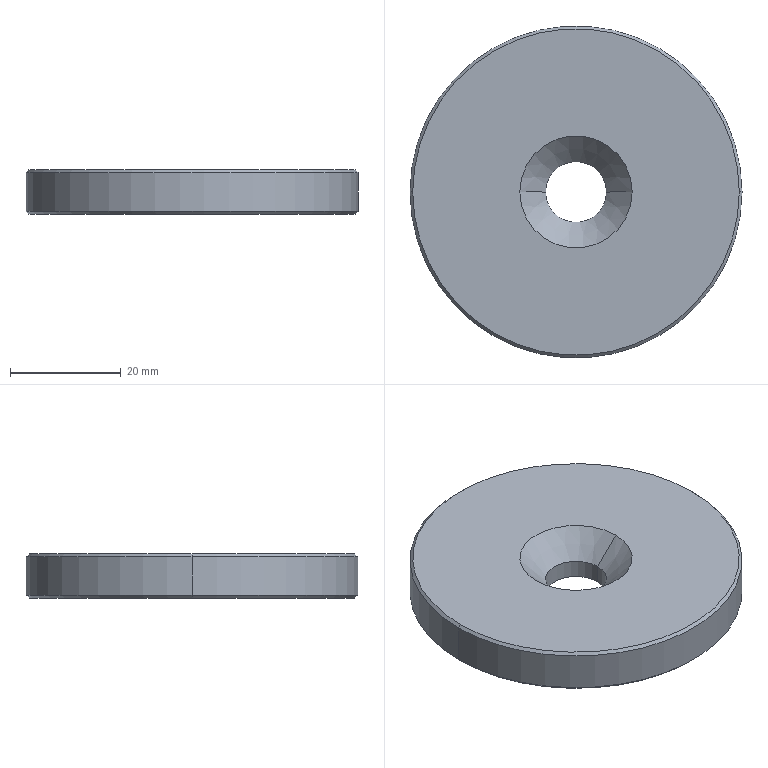Part | SolidWorks | features BaseBody 1 | 1 solid | 12 faces | box 60 x 60 x 8 mm | volume 21333 mm3 | cone 6 | cylinder 4 | plane 2 | commonest cylinder face diameters 11 x2 60 x2
STEP:
#1=CARTESIAN_POINT('',(-5.5,0.,3.35));
#2=VERTEX_POINT('',#1);
#3=CARTESIAN_POINT('',(5.5,0.,3.35));
#4=VERTEX_POINT('',#3);
#5=CARTESIAN_POINT('',(0.,0.,3.35));
#6=DIRECTION('',(0.,0.,1.));
#7=DIRECTION('',(1.,0.,0.));
#8=AXIS2_PLACEMENT_3D('',#5,#6,#7);
#9=CIRCLE('',#8,5.5);
#10=EDGE_CURVE('',#2,#4,#9,.T.);
#11=ORIENTED_EDGE('',*,*,#10,.F.);
#12=CARTESIAN_POINT('',(-10.15,0.,8.));
#13=VERTEX_POINT('',#12);
#14=CARTESIAN_POINT('',(-10.15,0.,8.));
#15=DIRECTION('',(-0.7071,0.,0.7071));
#16=VECTOR('',#15,1000.);
#17=LINE('',#14,#16);
#18=EDGE_CURVE('',#2,#13,#17,.T.);
#19=ORIENTED_EDGE('',*,*,#18,.T.);
#20=CARTESIAN_POINT('',(10.15,0.,8.));
#21=VERTEX_POINT('',#20);
#22=CARTESIAN_POINT('',(0.,0.,8.));
#23=DIRECTION('',(0.,0.,1.));
#24=DIRECTION('',(1.,0.,0.));
#25=AXIS2_PLACEMENT_3D('',#22,#23,#24);
#26=CIRCLE('',#25,10.15);
#27=EDGE_CURVE('',#13,#21,#26,.T.);
#28=ORIENTED_EDGE('',*,*,#27,.T.);
#29=CARTESIAN_POINT('',(10.15,0.,8.));
#30=DIRECTION('',(0.7071,0.,0.7071));
#31=VECTOR('',#30,1000.);
#32=LINE('',#29,#31);
#33=EDGE_CURVE('',#4,#21,#32,.T.);
#34=ORIENTED_EDGE('',*,*,#33,.F.);
#35=EDGE_LOOP('',(#11,#19,#28,#34));
#36=FACE_OUTER_BOUND('',#35,.T.);
#37=CARTESIAN_POINT('',(0.,0.,8.));
#38=DIRECTION('',(0.,0.,1.));
#39=DIRECTION('',(1.,0.,0.));
#40=AXIS2_PLACEMENT_3D('',#37,#38,#39);
#41=CONICAL_SURFACE('',#40,10.15,0.7854);
#42=ADVANCED_FACE('',(#36),#41,.F.);
#43=CARTESIAN_POINT('',(-5.5,0.,0.));
#44=VERTEX_POINT('',#43);
#45=CARTESIAN_POINT('',(5.5,0.,0.));
#46=VERTEX_POINT('',#45);
#47=CARTESIAN_POINT('',(0.,0.,0.));
#48=DIRECTION('',(0.,0.,1.));
#49=DIRECTION('',(1.,0.,0.));
#50=AXIS2_PLACEMENT_3D('',#47,#48,#49);
#51=CIRCLE('',#50,5.5);
#52=EDGE_CURVE('',#44,#46,#51,.T.);
#53=ORIENTED_EDGE('',*,*,#52,.F.);
#54=CARTESIAN_POINT('',(-5.5,0.,8.));
#55=DIRECTION('',(0.,0.,1.));
#56=VECTOR('',#55,1000.);
#57=LINE('',#54,#56);
#58=EDGE_CURVE('',#44,#2,#57,.T.);
#59=ORIENTED_EDGE('',*,*,#58,.T.);
#60=ORIENTED_EDGE('',*,*,#10,.T.);
#61=CARTESIAN_POINT('',(5.5,0.,8.));
#62=DIRECTION('',(0.,0.,1.));
#63=VECTOR('',#62,1000.);
#64=LINE('',#61,#63);
#65=EDGE_CURVE('',#46,#4,#64,.T.);
#66=ORIENTED_EDGE('',*,*,#65,.F.);
#67=EDGE_LOOP('',(#53,#59,#60,#66));
#68=FACE_OUTER_BOUND('',#67,.T.);
#69=CARTESIAN_POINT('',(0.,0.,8.));
#70=DIRECTION('',(0.,0.,1.));
#71=DIRECTION('',(1.,0.,0.));
#72=AXIS2_PLACEMENT_3D('',#69,#70,#71);
#73=CYLINDRICAL_SURFACE('',#72,5.5);
#74=ADVANCED_FACE('',(#68),#73,.F.);
#75=CARTESIAN_POINT('',(29.5,0.,8.));
#76=VERTEX_POINT('',#75);
#77=CARTESIAN_POINT('',(-29.5,0.,8.));
#78=VERTEX_POINT('',#77);
#79=CARTESIAN_POINT('',(0.,0.,8.));
#80=DIRECTION('',(0.,0.,1.));
#81=DIRECTION('',(1.,0.,0.));
#82=AXIS2_PLACEMENT_3D('',#79,#80,#81);
#83=CIRCLE('',#82,29.5);
#84=EDGE_CURVE('',#76,#78,#83,.T.);
#85=ORIENTED_EDGE('',*,*,#84,.F.);
#86=CARTESIAN_POINT('',(30.,0.,7.5));
#87=VERTEX_POINT('',#86);
#88=CARTESIAN_POINT('',(29.5,0.,8.));
#89=DIRECTION('',(0.7071,0.,-0.7071));
#90=VECTOR('',#89,1000.);
#91=LINE('',#88,#90);
#92=EDGE_CURVE('',#76,#87,#91,.T.);
#93=ORIENTED_EDGE('',*,*,#92,.T.);
#94=CARTESIAN_POINT('',(-30.,0.,7.5));
#95=VERTEX_POINT('',#94);
#96=CARTESIAN_POINT('',(0.,0.,7.5));
#97=DIRECTION('',(0.,0.,-1.));
#98=DIRECTION('',(1.,0.,0.));
#99=AXIS2_PLACEMENT_3D('',#96,#97,#98);
#100=CIRCLE('',#99,30.);
#101=EDGE_CURVE('',#95,#87,#100,.T.);
#102=ORIENTED_EDGE('',*,*,#101,.F.);
#103=CARTESIAN_POINT('',(-29.5,0.,8.));
#104=DIRECTION('',(-0.7071,0.,-0.7071));
#105=VECTOR('',#104,1000.);
#106=LINE('',#103,#105);
#107=EDGE_CURVE('',#78,#95,#106,.T.);
#108=ORIENTED_EDGE('',*,*,#107,.F.);
#109=EDGE_LOOP('',(#85,#93,#102,#108));
#110=FACE_OUTER_BOUND('',#109,.T.);
#111=CARTESIAN_POINT('',(0.,0.,8.));
#112=DIRECTION('',(0.,0.,-1.));
#113=DIRECTION('',(-1.,0.,0.));
#114=AXIS2_PLACEMENT_3D('',#111,#112,#113);
#115=CONICAL_SURFACE('',#114,29.5,0.7854);
#116=ADVANCED_FACE('',(#110),#115,.T.);
#117=CARTESIAN_POINT('',(-29.5,0.,0.));
#118=VERTEX_POINT('',#117);
#119=CARTESIAN_POINT('',(29.5,0.,0.));
#120=VERTEX_POINT('',#119);
#121=CARTESIAN_POINT('',(0.,0.,0.));
#122=DIRECTION('',(0.,0.,-1.));
#123=DIRECTION('',(1.,0.,0.));
#124=AXIS2_PLACEMENT_3D('',#121,#122,#123);
#125=CIRCLE('',#124,29.5);
#126=EDGE_CURVE('',#118,#120,#125,.T.);
#127=ORIENTED_EDGE('',*,*,#126,.F.);
#128=CARTESIAN_POINT('',(-30.,0.,0.5));
#129=VERTEX_POINT('',#128);
#130=CARTESIAN_POINT('',(-30.,0.,0.5));
#131=DIRECTION('',(-0.7071,0.,0.7071));
#132=VECTOR('',#131,1000.);
#133=LINE('',#130,#132);
#134=EDGE_CURVE('',#118,#129,#133,.T.);
#135=ORIENTED_EDGE('',*,*,#134,.T.);
#136=CARTESIAN_POINT('',(30.,0.,0.5));
#137=VERTEX_POINT('',#136);
#138=CARTESIAN_POINT('',(0.,0.,0.5));
#139=DIRECTION('',(0.,0.,1.));
#140=DIRECTION('',(1.,0.,0.));
#141=AXIS2_PLACEMENT_3D('',#138,#139,#140);
#142=CIRCLE('',#141,30.);
#143=EDGE_CURVE('',#137,#129,#142,.T.);
#144=ORIENTED_EDGE('',*,*,#143,.F.);
#145=CARTESIAN_POINT('',(30.,0.,0.5));
#146=DIRECTION('',(0.7071,0.,0.7071));
#147=VECTOR('',#146,1000.);
#148=LINE('',#145,#147);
#149=EDGE_CURVE('',#120,#137,#148,.T.);
#150=ORIENTED_EDGE('',*,*,#149,.F.);
#151=EDGE_LOOP('',(#127,#135,#144,#150));
#152=FACE_OUTER_BOUND('',#151,.T.);
#153=CARTESIAN_POINT('',(0.,0.,0.5));
#154=DIRECTION('',(0.,0.,1.));
#155=DIRECTION('',(1.,0.,0.));
#156=AXIS2_PLACEMENT_3D('',#153,#154,#155);
#157=CONICAL_SURFACE('',#156,30.,0.7854);
#158=ADVANCED_FACE('',(#152),#157,.T.);
#159=ORIENTED_EDGE('',*,*,#101,.T.);
#160=CARTESIAN_POINT('',(30.,0.,8.));
#161=DIRECTION('',(0.,0.,-1.));
#162=VECTOR('',#161,1000.);
#163=LINE('',#160,#162);
#164=EDGE_CURVE('',#87,#137,#163,.T.);
#165=ORIENTED_EDGE('',*,*,#164,.T.);
#166=ORIENTED_EDGE('',*,*,#143,.T.);
#167=CARTESIAN_POINT('',(-30.,0.,8.));
#168=DIRECTION('',(0.,0.,-1.));
#169=VECTOR('',#168,1000.);
#170=LINE('',#167,#169);
#171=EDGE_CURVE('',#95,#129,#170,.T.);
#172=ORIENTED_EDGE('',*,*,#171,.F.);
#173=EDGE_LOOP('',(#159,#165,#166,#172));
#174=FACE_OUTER_BOUND('',#173,.T.);
#175=CARTESIAN_POINT('',(0.,0.,8.));
#176=DIRECTION('',(0.,0.,-1.));
#177=DIRECTION('',(-1.,0.,0.));
#178=AXIS2_PLACEMENT_3D('',#175,#176,#177);
#179=CYLINDRICAL_SURFACE('',#178,30.);
#180=ADVANCED_FACE('',(#174),#179,.T.);
#181=ORIENTED_EDGE('',*,*,#164,.F.);
#182=CARTESIAN_POINT('',(0.,0.,7.5));
#183=DIRECTION('',(0.,0.,-1.));
#184=DIRECTION('',(1.,0.,0.));
#185=AXIS2_PLACEMENT_3D('',#182,#183,#184);
#186=CIRCLE('',#185,30.);
#187=EDGE_CURVE('',#87,#95,#186,.T.);
#188=ORIENTED_EDGE('',*,*,#187,.T.);
#189=ORIENTED_EDGE('',*,*,#171,.T.);
#190=CARTESIAN_POINT('',(0.,0.,0.5));
#191=DIRECTION('',(0.,0.,1.));
#192=DIRECTION('',(1.,0.,0.));
#193=AXIS2_PLACEMENT_3D('',#190,#191,#192);
#194=CIRCLE('',#193,30.);
#195=EDGE_CURVE('',#129,#137,#194,.T.);
#196=ORIENTED_EDGE('',*,*,#195,.T.);
#197=EDGE_LOOP('',(#181,#188,#189,#196));
#198=FACE_OUTER_BOUND('',#197,.T.);
#199=CARTESIAN_POINT('',(0.,0.,8.));
#200=DIRECTION('',(0.,0.,-1.));
#201=DIRECTION('',(-1.,0.,0.));
#202=AXIS2_PLACEMENT_3D('',#199,#200,#201);
#203=CYLINDRICAL_SURFACE('',#202,30.);
#204=ADVANCED_FACE('',(#198),#203,.T.);
#205=CARTESIAN_POINT('',(0.,0.,8.));
#206=DIRECTION('',(0.,0.,1.));
#207=DIRECTION('',(1.,0.,0.));
#208=AXIS2_PLACEMENT_3D('',#205,#206,#207);
#209=CIRCLE('',#208,10.15);
#210=EDGE_CURVE('',#21,#13,#209,.T.);
#211=ORIENTED_EDGE('',*,*,#210,.F.);
#212=ORIENTED_EDGE('',*,*,#27,.F.);
#213=EDGE_LOOP('',(#211,#212));
#214=FACE_BOUND('',#213,.T.);
#215=CARTESIAN_POINT('',(0.,0.,8.));
#216=DIRECTION('',(0.,0.,1.));
#217=DIRECTION('',(1.,0.,0.));
#218=AXIS2_PLACEMENT_3D('',#215,#216,#217);
#219=CIRCLE('',#218,29.5);
#220=EDGE_CURVE('',#78,#76,#219,.T.);
#221=ORIENTED_EDGE('',*,*,#220,.T.);
#222=ORIENTED_EDGE('',*,*,#84,.T.);
#223=EDGE_LOOP('',(#221,#222));
#224=FACE_OUTER_BOUND('',#223,.T.);
#225=CARTESIAN_POINT('',(0.,0.,8.));
#226=DIRECTION('',(0.,0.,1.));
#227=DIRECTION('',(1.,0.,0.));
#228=AXIS2_PLACEMENT_3D('',#225,#226,#227);
#229=PLANE('',#228);
#230=ADVANCED_FACE('',(#214,#224),#229,.T.);
#231=CARTESIAN_POINT('',(0.,0.,0.));
#232=DIRECTION('',(0.,0.,1.));
#233=DIRECTION('',(1.,0.,0.));
#234=AXIS2_PLACEMENT_3D('',#231,#232,#233);
#235=CIRCLE('',#234,5.5);
#236=EDGE_CURVE('',#46,#44,#235,.T.);
#237=ORIENTED_EDGE('',*,*,#236,.T.);
#238=ORIENTED_EDGE('',*,*,#52,.T.);
#239=EDGE_LOOP('',(#237,#238));
#240=FACE_BOUND('',#239,.T.);
#241=CARTESIAN_POINT('',(0.,0.,0.));
#242=DIRECTION('',(0.,0.,-1.));
#243=DIRECTION('',(1.,0.,0.));
#244=AXIS2_PLACEMENT_3D('',#241,#242,#243);
#245=CIRCLE('',#244,29.5);
#246=EDGE_CURVE('',#120,#118,#245,.T.);
#247=ORIENTED_EDGE('',*,*,#246,.T.);
#248=ORIENTED_EDGE('',*,*,#126,.T.);
#249=EDGE_LOOP('',(#247,#248));
#250=FACE_OUTER_BOUND('',#249,.T.);
#251=CARTESIAN_POINT('',(0.,0.,0.));
#252=DIRECTION('',(0.,0.,1.));
#253=DIRECTION('',(1.,0.,0.));
#254=AXIS2_PLACEMENT_3D('',#251,#252,#253);
#255=PLANE('',#254);
#256=ADVANCED_FACE('',(#240,#250),#255,.F.);
#257=ORIENTED_EDGE('',*,*,#134,.F.);
#258=ORIENTED_EDGE('',*,*,#246,.F.);
#259=ORIENTED_EDGE('',*,*,#149,.T.);
#260=ORIENTED_EDGE('',*,*,#195,.F.);
#261=EDGE_LOOP('',(#257,#258,#259,#260));
#262=FACE_OUTER_BOUND('',#261,.T.);
#263=CARTESIAN_POINT('',(0.,0.,0.5));
#264=DIRECTION('',(0.,0.,1.));
#265=DIRECTION('',(1.,0.,0.));
#266=AXIS2_PLACEMENT_3D('',#263,#264,#265);
#267=CONICAL_SURFACE('',#266,30.,0.7854);
#268=ADVANCED_FACE('',(#262),#267,.T.);
#269=ORIENTED_EDGE('',*,*,#92,.F.);
#270=ORIENTED_EDGE('',*,*,#220,.F.);
#271=ORIENTED_EDGE('',*,*,#107,.T.);
#272=ORIENTED_EDGE('',*,*,#187,.F.);
#273=EDGE_LOOP('',(#269,#270,#271,#272));
#274=FACE_OUTER_BOUND('',#273,.T.);
#275=CARTESIAN_POINT('',(0.,0.,8.));
#276=DIRECTION('',(0.,0.,-1.));
#277=DIRECTION('',(-1.,0.,0.));
#278=AXIS2_PLACEMENT_3D('',#275,#276,#277);
#279=CONICAL_SURFACE('',#278,29.5,0.7854);
#280=ADVANCED_FACE('',(#274),#279,.T.);
#281=ORIENTED_EDGE('',*,*,#58,.F.);
#282=ORIENTED_EDGE('',*,*,#236,.F.);
#283=ORIENTED_EDGE('',*,*,#65,.T.);
#284=CARTESIAN_POINT('',(0.,0.,3.35));
#285=DIRECTION('',(0.,0.,1.));
#286=DIRECTION('',(1.,0.,0.));
#287=AXIS2_PLACEMENT_3D('',#284,#285,#286);
#288=CIRCLE('',#287,5.5);
#289=EDGE_CURVE('',#4,#2,#288,.T.);
#290=ORIENTED_EDGE('',*,*,#289,.T.);
#291=EDGE_LOOP('',(#281,#282,#283,#290));
#292=FACE_OUTER_BOUND('',#291,.T.);
#293=CARTESIAN_POINT('',(0.,0.,8.));
#294=DIRECTION('',(0.,0.,1.));
#295=DIRECTION('',(1.,0.,0.));
#296=AXIS2_PLACEMENT_3D('',#293,#294,#295);
#297=CYLINDRICAL_SURFACE('',#296,5.5);
#298=ADVANCED_FACE('',(#292),#297,.F.);
#299=ORIENTED_EDGE('',*,*,#18,.F.);
#300=ORIENTED_EDGE('',*,*,#289,.F.);
#301=ORIENTED_EDGE('',*,*,#33,.T.);
#302=ORIENTED_EDGE('',*,*,#210,.T.);
#303=EDGE_LOOP('',(#299,#300,#301,#302));
#304=FACE_OUTER_BOUND('',#303,.T.);
#305=CARTESIAN_POINT('',(0.,0.,8.));
#306=DIRECTION('',(0.,0.,1.));
#307=DIRECTION('',(1.,0.,0.));
#308=AXIS2_PLACEMENT_3D('',#305,#306,#307);
#309=CONICAL_SURFACE('',#308,10.15,0.7854);
#310=ADVANCED_FACE('',(#304),#309,.F.);
#311=CLOSED_SHELL('',(#42,#74,#116,#158,#180,#204,#230,#256,#268,#280,#298,#310));
#312=MANIFOLD_SOLID_BREP('',#311);
#313=CARTESIAN_POINT('',(0.,0.,0.));
#314=DIRECTION('',(0.,0.,1.));
#315=DIRECTION('',(1.,0.,0.));
#316=AXIS2_PLACEMENT_3D('',#313,#314,#315);
#317=(LENGTH_UNIT()NAMED_UNIT(*)SI_UNIT(.MILLI.,.METRE.));
#318=UNCERTAINTY_MEASURE_WITH_UNIT(LENGTH_MEASURE(0.00001),#317,'','');
#319=(NAMED_UNIT(*)PLANE_ANGLE_UNIT()SI_UNIT($,.RADIAN.));
#320=(NAMED_UNIT(*)SI_UNIT($,.STERADIAN.)SOLID_ANGLE_UNIT());
#321=(GEOMETRIC_REPRESENTATION_CONTEXT(3)GLOBAL_UNCERTAINTY_ASSIGNED_CONTEXT((#318))GLOBAL_UNIT_ASSIGNED_CONTEXT((#317,#319,#320))REPRESENTATION_CONTEXT('',''));
#322=ADVANCED_BREP_SHAPE_REPRESENTATION('',(#312,#316),#321);